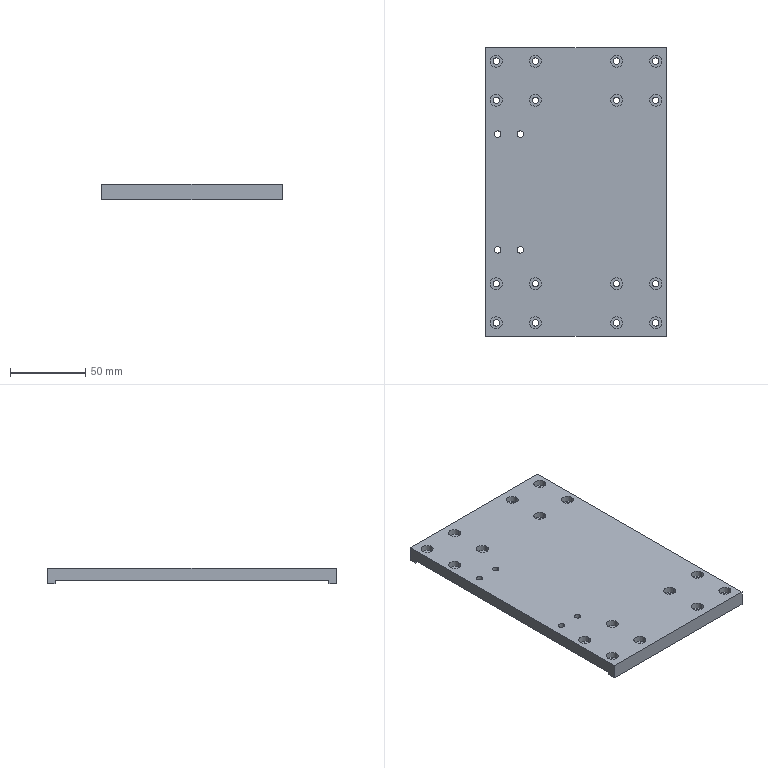Part | Creo | features CURVE 3, DATUM PLANE 3, PROTRUSION 2, COORDINATE SYSTEM 1, CUT 1 | 1 solid | 98 faces | box 120 x 192 x 10 mm | volume 182173 mm3 | cylinder 72 | plane 26 | commonest cylinder face diameters 4.2 x40 8 x32